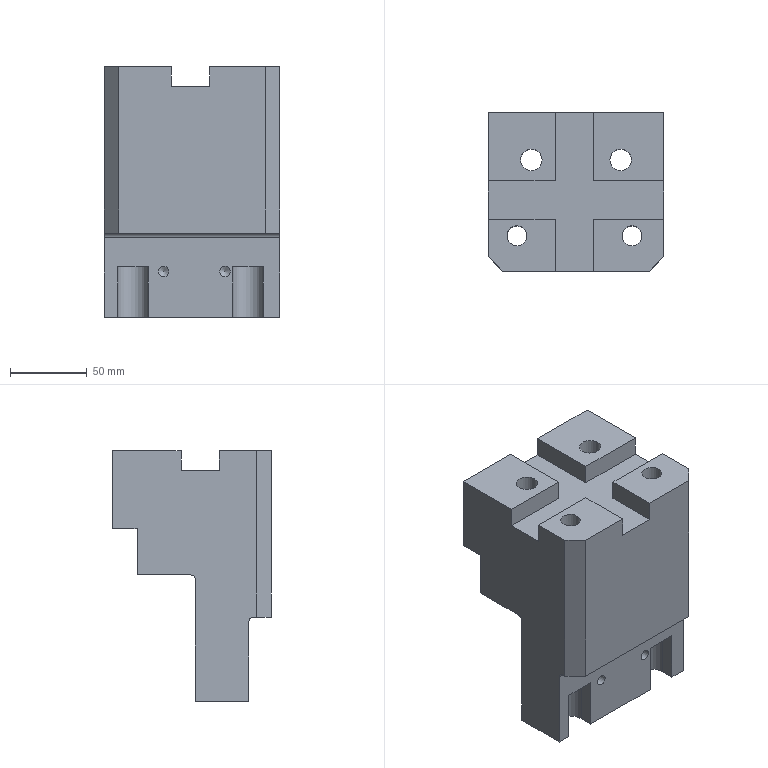Part | STEP file | 1_id158_x_t | 1 solid | 81 faces | box 114.3 x 103.32 x 163.553 mm | volume 1068364 mm3 | plane 50 | cylinder 26 | cone 5 | commonest cylinder face diameters 6 x10 6.75 x4 20 x4 3.3 x2 6.8 x2 13 x2